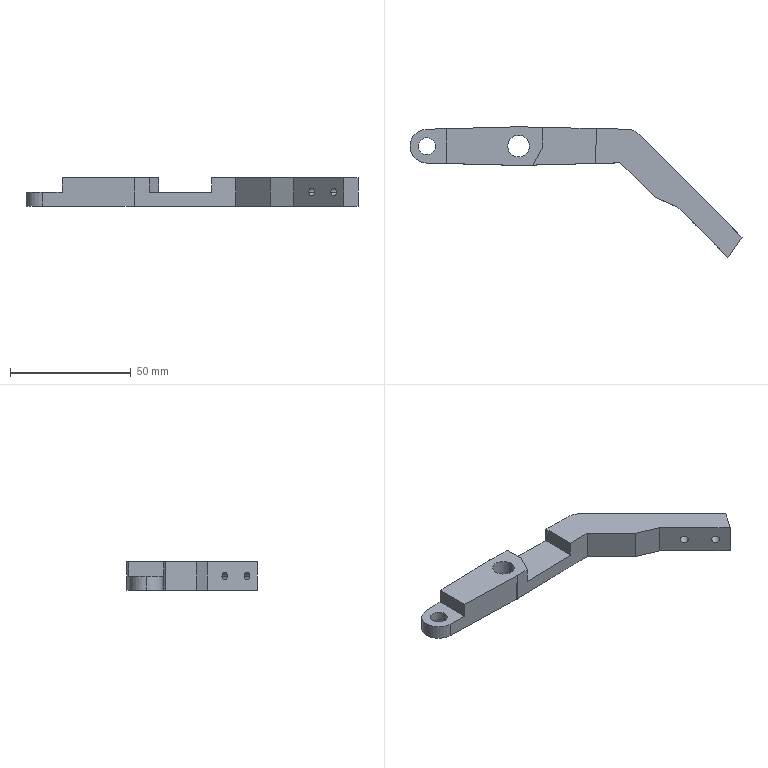Part | STEP file | Ngam kep 2 | 1 solid | 34 faces | box 137.617 x 54.035 x 11.8 mm | volume 19679 mm3 | plane 19 | cylinder 15 | commonest cylinder face diameters 3.3 x4 9 x4 14 x3 7 x2 16 x2